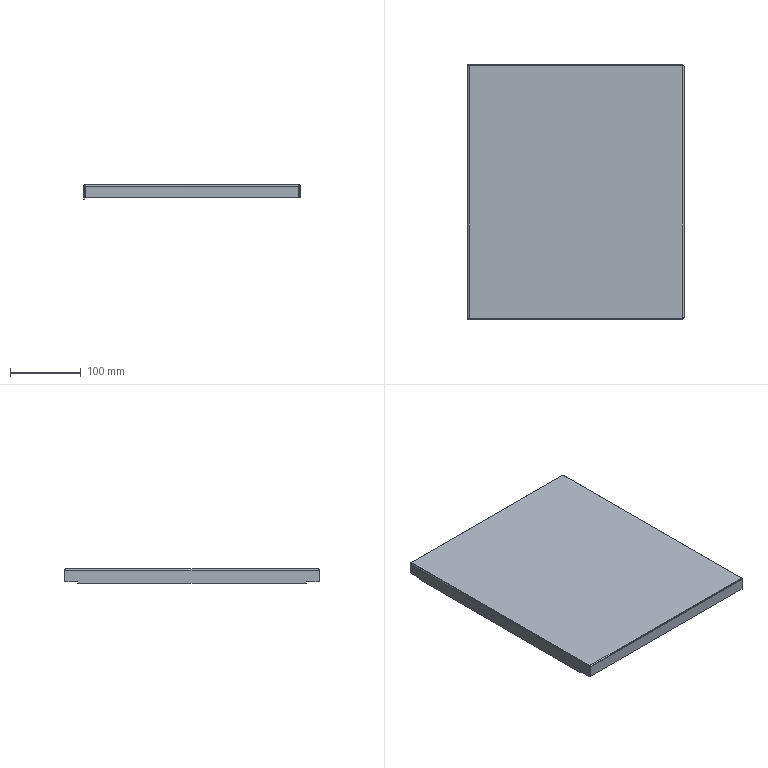Part | SolidWorks | features BaseBody 1 | 1 solid | 44 faces | box 304.9 x 358.65 x 20 mm | volume 157769 mm3 | plane 32 | cylinder 8 | spline 4 | commonest cylinder face diameters 1 x4 3.4 x4
STEP:
#1=CARTESIAN_POINT('',(-152.45,-179.325,-18.));
#2=VERTEX_POINT('',#1);
#3=CARTESIAN_POINT('',(-152.45,-161.325,-18.));
#4=VERTEX_POINT('',#3);
#5=CARTESIAN_POINT('',(-152.45,-179.325,-18.));
#6=DIRECTION('',(0.,1.,0.));
#7=VECTOR('',#6,1000.);
#8=LINE('',#5,#7);
#9=EDGE_CURVE('',#2,#4,#8,.T.);
#10=ORIENTED_EDGE('',*,*,#9,.T.);
#11=CARTESIAN_POINT('',(-151.25,-161.325,-18.));
#12=VERTEX_POINT('',#11);
#13=CARTESIAN_POINT('',(-151.25,-161.325,-18.));
#14=DIRECTION('',(-1.,0.,0.));
#15=VECTOR('',#14,1000.);
#16=LINE('',#13,#15);
#17=EDGE_CURVE('',#12,#4,#16,.T.);
#18=ORIENTED_EDGE('',*,*,#17,.F.);
#19=CARTESIAN_POINT('',(-151.25,-179.325,-18.));
#20=VERTEX_POINT('',#19);
#21=CARTESIAN_POINT('',(-151.25,-179.325,-18.));
#22=DIRECTION('',(0.,1.,0.));
#23=VECTOR('',#22,1000.);
#24=LINE('',#21,#23);
#25=EDGE_CURVE('',#20,#12,#24,.T.);
#26=ORIENTED_EDGE('',*,*,#25,.F.);
#27=CARTESIAN_POINT('',(-151.25,-179.325,-18.));
#28=DIRECTION('',(-1.,0.,0.));
#29=VECTOR('',#28,1000.);
#30=LINE('',#27,#29);
#31=EDGE_CURVE('',#20,#2,#30,.T.);
#32=ORIENTED_EDGE('',*,*,#31,.T.);
#33=EDGE_LOOP('',(#10,#18,#26,#32));
#34=FACE_OUTER_BOUND('',#33,.T.);
#35=CARTESIAN_POINT('',(-151.25,-179.325,-18.));
#36=DIRECTION('',(0.,0.,1.));
#37=DIRECTION('',(1.,0.,0.));
#38=AXIS2_PLACEMENT_3D('',#35,#36,#37);
#39=PLANE('',#38);
#40=ADVANCED_FACE('',(#34),#39,.F.);
#41=CARTESIAN_POINT('',(-152.45,-161.325,-20.));
#42=VERTEX_POINT('',#41);
#43=CARTESIAN_POINT('',(-152.45,-161.325,-20.));
#44=DIRECTION('',(0.,0.,-1.));
#45=VECTOR('',#44,1000.);
#46=LINE('',#43,#45);
#47=EDGE_CURVE('',#4,#42,#46,.T.);
#48=ORIENTED_EDGE('',*,*,#47,.T.);
#49=CARTESIAN_POINT('',(-151.25,-161.325,-20.));
#50=VERTEX_POINT('',#49);
#51=CARTESIAN_POINT('',(-151.25,-161.325,-20.));
#52=DIRECTION('',(-1.,0.,0.));
#53=VECTOR('',#52,1000.);
#54=LINE('',#51,#53);
#55=EDGE_CURVE('',#50,#42,#54,.T.);
#56=ORIENTED_EDGE('',*,*,#55,.F.);
#57=CARTESIAN_POINT('',(-151.25,-161.325,-20.));
#58=DIRECTION('',(0.,0.,-1.));
#59=VECTOR('',#58,1000.);
#60=LINE('',#57,#59);
#61=EDGE_CURVE('',#12,#50,#60,.T.);
#62=ORIENTED_EDGE('',*,*,#61,.F.);
#63=ORIENTED_EDGE('',*,*,#17,.T.);
#64=EDGE_LOOP('',(#48,#56,#62,#63));
#65=FACE_OUTER_BOUND('',#64,.T.);
#66=CARTESIAN_POINT('',(-151.25,-161.325,-20.));
#67=DIRECTION('',(0.,1.,0.));
#68=DIRECTION('',(1.,0.,0.));
#69=AXIS2_PLACEMENT_3D('',#66,#67,#68);
#70=PLANE('',#69);
#71=ADVANCED_FACE('',(#65),#70,.F.);
#72=CARTESIAN_POINT('',(-152.45,161.325,-20.));
#73=VERTEX_POINT('',#72);
#74=CARTESIAN_POINT('',(-152.45,161.325,-18.));
#75=VERTEX_POINT('',#74);
#76=CARTESIAN_POINT('',(-152.45,161.325,-20.));
#77=DIRECTION('',(0.,0.,1.));
#78=VECTOR('',#77,1000.);
#79=LINE('',#76,#78);
#80=EDGE_CURVE('',#73,#75,#79,.T.);
#81=ORIENTED_EDGE('',*,*,#80,.T.);
#82=CARTESIAN_POINT('',(-151.25,161.325,-18.));
#83=VERTEX_POINT('',#82);
#84=CARTESIAN_POINT('',(-151.25,161.325,-18.));
#85=DIRECTION('',(-1.,0.,0.));
#86=VECTOR('',#85,1000.);
#87=LINE('',#84,#86);
#88=EDGE_CURVE('',#83,#75,#87,.T.);
#89=ORIENTED_EDGE('',*,*,#88,.F.);
#90=CARTESIAN_POINT('',(-151.25,161.325,-20.));
#91=VERTEX_POINT('',#90);
#92=CARTESIAN_POINT('',(-151.25,161.325,-20.));
#93=DIRECTION('',(0.,0.,1.));
#94=VECTOR('',#93,1000.);
#95=LINE('',#92,#94);
#96=EDGE_CURVE('',#91,#83,#95,.T.);
#97=ORIENTED_EDGE('',*,*,#96,.F.);
#98=CARTESIAN_POINT('',(-151.25,161.325,-20.));
#99=DIRECTION('',(-1.,0.,0.));
#100=VECTOR('',#99,1000.);
#101=LINE('',#98,#100);
#102=EDGE_CURVE('',#91,#73,#101,.T.);
#103=ORIENTED_EDGE('',*,*,#102,.T.);
#104=EDGE_LOOP('',(#81,#89,#97,#103));
#105=FACE_OUTER_BOUND('',#104,.T.);
#106=CARTESIAN_POINT('',(-151.25,161.325,-20.));
#107=DIRECTION('',(0.,-1.,0.));
#108=DIRECTION('',(0.,0.,-1.));
#109=AXIS2_PLACEMENT_3D('',#106,#107,#108);
#110=PLANE('',#109);
#111=ADVANCED_FACE('',(#105),#110,.F.);
#112=CARTESIAN_POINT('',(-152.45,179.325,-18.));
#113=VERTEX_POINT('',#112);
#114=CARTESIAN_POINT('',(-152.45,179.325,-18.));
#115=DIRECTION('',(0.,1.,0.));
#116=VECTOR('',#115,1000.);
#117=LINE('',#114,#116);
#118=EDGE_CURVE('',#75,#113,#117,.T.);
#119=ORIENTED_EDGE('',*,*,#118,.T.);
#120=CARTESIAN_POINT('',(-151.25,179.325,-18.));
#121=VERTEX_POINT('',#120);
#122=CARTESIAN_POINT('',(-151.25,179.325,-18.));
#123=DIRECTION('',(-1.,0.,0.));
#124=VECTOR('',#123,1000.);
#125=LINE('',#122,#124);
#126=EDGE_CURVE('',#121,#113,#125,.T.);
#127=ORIENTED_EDGE('',*,*,#126,.F.);
#128=CARTESIAN_POINT('',(-151.25,179.325,-18.));
#129=DIRECTION('',(0.,1.,0.));
#130=VECTOR('',#129,1000.);
#131=LINE('',#128,#130);
#132=EDGE_CURVE('',#83,#121,#131,.T.);
#133=ORIENTED_EDGE('',*,*,#132,.F.);
#134=ORIENTED_EDGE('',*,*,#88,.T.);
#135=EDGE_LOOP('',(#119,#127,#133,#134));
#136=FACE_OUTER_BOUND('',#135,.T.);
#137=CARTESIAN_POINT('',(-151.25,179.325,-18.));
#138=DIRECTION('',(0.,0.,1.));
#139=DIRECTION('',(1.,0.,0.));
#140=AXIS2_PLACEMENT_3D('',#137,#138,#139);
#141=PLANE('',#140);
#142=ADVANCED_FACE('',(#136),#141,.F.);
#143=CARTESIAN_POINT('',(150.543,179.325,-18.));
#144=VERTEX_POINT('',#143);
#145=CARTESIAN_POINT('',(150.543,178.125,-18.));
#146=VERTEX_POINT('',#145);
#147=CARTESIAN_POINT('',(150.543,179.325,-18.));
#148=DIRECTION('',(0.,-1.,0.));
#149=VECTOR('',#148,1000.);
#150=LINE('',#147,#149);
#151=EDGE_CURVE('',#144,#146,#150,.T.);
#152=ORIENTED_EDGE('',*,*,#151,.F.);
#153=CARTESIAN_POINT('',(150.543,179.325,-1.7));
#154=VERTEX_POINT('',#153);
#155=CARTESIAN_POINT('',(150.543,179.325,0.));
#156=DIRECTION('',(0.,0.,-1.));
#157=VECTOR('',#156,1000.);
#158=LINE('',#155,#157);
#159=EDGE_CURVE('',#154,#144,#158,.T.);
#160=ORIENTED_EDGE('',*,*,#159,.F.);
#161=CARTESIAN_POINT('',(150.543,178.125,-1.7));
#162=VERTEX_POINT('',#161);
#163=CARTESIAN_POINT('',(150.543,178.125,-1.7));
#164=DIRECTION('',(0.,-1.,0.));
#165=VECTOR('',#164,1000.);
#166=LINE('',#163,#165);
#167=EDGE_CURVE('',#154,#162,#166,.T.);
#168=ORIENTED_EDGE('',*,*,#167,.T.);
#169=CARTESIAN_POINT('',(150.543,178.125,-1.2));
#170=DIRECTION('',(0.,0.,-1.));
#171=VECTOR('',#170,1000.);
#172=LINE('',#169,#171);
#173=EDGE_CURVE('',#162,#146,#172,.T.);
#174=ORIENTED_EDGE('',*,*,#173,.T.);
#175=EDGE_LOOP('',(#152,#160,#168,#174));
#176=FACE_OUTER_BOUND('',#175,.T.);
#177=CARTESIAN_POINT('',(150.543,178.125,-1.2));
#178=DIRECTION('',(-1.,0.,0.));
#179=DIRECTION('',(0.,0.,1.));
#180=AXIS2_PLACEMENT_3D('',#177,#178,#179);
#181=PLANE('',#180);
#182=ADVANCED_FACE('',(#176),#181,.F.);
#183=CARTESIAN_POINT('',(-150.75,179.325,-18.));
#184=VERTEX_POINT('',#183);
#185=CARTESIAN_POINT('',(0.,179.325,-18.));
#186=DIRECTION('',(-1.,0.,0.));
#187=VECTOR('',#186,1000.);
#188=LINE('',#185,#187);
#189=EDGE_CURVE('',#144,#184,#188,.T.);
#190=ORIENTED_EDGE('',*,*,#189,.F.);
#191=ORIENTED_EDGE('',*,*,#151,.T.);
#192=CARTESIAN_POINT('',(-150.75,178.125,-18.));
#193=VERTEX_POINT('',#192);
#194=CARTESIAN_POINT('',(-150.75,178.125,-18.));
#195=DIRECTION('',(-1.,0.,0.));
#196=VECTOR('',#195,1000.);
#197=LINE('',#194,#196);
#198=EDGE_CURVE('',#146,#193,#197,.T.);
#199=ORIENTED_EDGE('',*,*,#198,.T.);
#200=CARTESIAN_POINT('',(-150.75,179.325,-18.));
#201=DIRECTION('',(0.,-1.,0.));
#202=VECTOR('',#201,1000.);
#203=LINE('',#200,#202);
#204=EDGE_CURVE('',#184,#193,#203,.T.);
#205=ORIENTED_EDGE('',*,*,#204,.F.);
#206=EDGE_LOOP('',(#190,#191,#199,#205));
#207=FACE_OUTER_BOUND('',#206,.T.);
#208=CARTESIAN_POINT('',(-150.75,179.325,-18.));
#209=DIRECTION('',(0.,0.,1.));
#210=DIRECTION('',(0.,-1.,0.));
#211=AXIS2_PLACEMENT_3D('',#208,#209,#210);
#212=PLANE('',#211);
#213=ADVANCED_FACE('',(#207),#212,.F.);
#214=ORIENTED_EDGE('',*,*,#173,.F.);
#215=CARTESIAN_POINT('',(-150.75,178.125,-1.7));
#216=VERTEX_POINT('',#215);
#217=CARTESIAN_POINT('',(-150.75,178.125,-1.7));
#218=DIRECTION('',(1.,0.,0.));
#219=VECTOR('',#218,1000.);
#220=LINE('',#217,#219);
#221=EDGE_CURVE('',#216,#162,#220,.T.);
#222=ORIENTED_EDGE('',*,*,#221,.F.);
#223=CARTESIAN_POINT('',(-150.75,178.125,-1.2));
#224=DIRECTION('',(0.,0.,1.));
#225=VECTOR('',#224,1000.);
#226=LINE('',#223,#225);
#227=EDGE_CURVE('',#193,#216,#226,.T.);
#228=ORIENTED_EDGE('',*,*,#227,.F.);
#229=ORIENTED_EDGE('',*,*,#198,.F.);
#230=EDGE_LOOP('',(#214,#222,#228,#229));
#231=FACE_OUTER_BOUND('',#230,.T.);
#232=CARTESIAN_POINT('',(0.,178.125,0.));
#233=DIRECTION('',(0.,-1.,0.));
#234=DIRECTION('',(0.,0.,-1.));
#235=AXIS2_PLACEMENT_3D('',#232,#233,#234);
#236=PLANE('',#235);
#237=ADVANCED_FACE('',(#231),#236,.T.);
#238=CARTESIAN_POINT('',(-150.75,179.325,-1.7));
#239=VERTEX_POINT('',#238);
#240=CARTESIAN_POINT('',(-150.75,179.325,-1.7));
#241=DIRECTION('',(-1.,0.,0.));
#242=VECTOR('',#241,1000.);
#243=LINE('',#240,#242);
#244=EDGE_CURVE('',#154,#239,#243,.T.);
#245=ORIENTED_EDGE('',*,*,#244,.F.);
#246=ORIENTED_EDGE('',*,*,#159,.T.);
#247=ORIENTED_EDGE('',*,*,#189,.T.);
#248=CARTESIAN_POINT('',(-150.75,179.325,0.));
#249=DIRECTION('',(0.,0.,1.));
#250=VECTOR('',#249,1000.);
#251=LINE('',#248,#250);
#252=EDGE_CURVE('',#184,#239,#251,.T.);
#253=ORIENTED_EDGE('',*,*,#252,.T.);
#254=EDGE_LOOP('',(#245,#246,#247,#253));
#255=FACE_OUTER_BOUND('',#254,.T.);
#256=CARTESIAN_POINT('',(0.,179.325,0.));
#257=DIRECTION('',(0.,-1.,0.));
#258=DIRECTION('',(0.,0.,-1.));
#259=AXIS2_PLACEMENT_3D('',#256,#257,#258);
#260=PLANE('',#259);
#261=ADVANCED_FACE('',(#255),#260,.F.);
#262=CARTESIAN_POINT('',(-150.75,179.325,-1.7));
#263=DIRECTION('',(0.,1.,0.));
#264=VECTOR('',#263,1000.);
#265=LINE('',#262,#264);
#266=EDGE_CURVE('',#216,#239,#265,.T.);
#267=ORIENTED_EDGE('',*,*,#266,.T.);
#268=ORIENTED_EDGE('',*,*,#252,.F.);
#269=ORIENTED_EDGE('',*,*,#204,.T.);
#270=ORIENTED_EDGE('',*,*,#227,.T.);
#271=EDGE_LOOP('',(#267,#268,#269,#270));
#272=FACE_OUTER_BOUND('',#271,.T.);
#273=CARTESIAN_POINT('',(-150.75,179.325,-1.2));
#274=DIRECTION('',(1.,0.,0.));
#275=DIRECTION('',(0.,0.,-1.));
#276=AXIS2_PLACEMENT_3D('',#273,#274,#275);
#277=PLANE('',#276);
#278=ADVANCED_FACE('',(#272),#277,.F.);
#279=CARTESIAN_POINT('',(150.75,177.625,-1.2));
#280=VERTEX_POINT('',#279);
#281=CARTESIAN_POINT('',(-150.75,177.625,-1.2));
#282=VERTEX_POINT('',#281);
#283=CARTESIAN_POINT('',(150.75,177.625,-1.2));
#284=DIRECTION('',(-1.,0.,0.));
#285=VECTOR('',#284,1000.);
#286=LINE('',#283,#285);
#287=EDGE_CURVE('',#280,#282,#286,.T.);
#288=ORIENTED_EDGE('',*,*,#287,.T.);
#289=CARTESIAN_POINT('',(-150.75,177.625,-1.7));
#290=DIRECTION('',(-1.,0.,0.));
#291=DIRECTION('',(0.,0.,-1.));
#292=AXIS2_PLACEMENT_3D('',#289,#290,#291);
#293=CIRCLE('',#292,0.5);
#294=EDGE_CURVE('',#282,#216,#293,.T.);
#295=ORIENTED_EDGE('',*,*,#294,.T.);
#296=ORIENTED_EDGE('',*,*,#221,.T.);
#297=CARTESIAN_POINT('',(150.543,178.125,-1.7));
#298=CARTESIAN_POINT('',(150.577,178.125,-1.569));
#299=CARTESIAN_POINT('',(150.612,178.071,-1.439));
#300=CARTESIAN_POINT('',(150.681,177.886,-1.254));
#301=CARTESIAN_POINT('',(150.715,177.756,-1.2));
#302=CARTESIAN_POINT('',(150.75,177.625,-1.2));
#303=B_SPLINE_CURVE_WITH_KNOTS('',3,(#297,#298,#299,#300,#301,#302),.UNSPECIFIED.,.F.,.F.,(4,2,4),(0.,0.5,1.),.UNSPECIFIED.);
#304=EDGE_CURVE('',#162,#280,#303,.T.);
#305=ORIENTED_EDGE('',*,*,#304,.T.);
#306=EDGE_LOOP('',(#288,#295,#296,#305));
#307=FACE_OUTER_BOUND('',#306,.T.);
#308=CARTESIAN_POINT('',(150.75,177.625,-1.7));
#309=DIRECTION('',(1.,0.,0.));
#310=DIRECTION('',(0.,1.,0.));
#311=AXIS2_PLACEMENT_3D('',#308,#309,#310);
#312=CYLINDRICAL_SURFACE('',#311,0.5);
#313=ADVANCED_FACE('',(#307),#312,.F.);
#314=CARTESIAN_POINT('',(150.75,177.625,0.));
#315=VERTEX_POINT('',#314);
#316=CARTESIAN_POINT('',(-150.75,177.625,0.));
#317=VERTEX_POINT('',#316);
#318=CARTESIAN_POINT('',(150.75,177.625,0.));
#319=DIRECTION('',(-1.,0.,0.));
#320=VECTOR('',#319,1000.);
#321=LINE('',#318,#320);
#322=EDGE_CURVE('',#315,#317,#321,.T.);
#323=ORIENTED_EDGE('',*,*,#322,.F.);
#324=CARTESIAN_POINT('',(150.543,179.325,-1.7));
#325=CARTESIAN_POINT('',(150.56,179.325,-1.477));
#326=CARTESIAN_POINT('',(150.577,179.281,-1.255));
#327=CARTESIAN_POINT('',(150.612,179.11,-0.8438));
#328=CARTESIAN_POINT('',(150.629,178.984,-0.6553));
#329=CARTESIAN_POINT('',(150.664,178.67,-0.3406));
#330=CARTESIAN_POINT('',(150.681,178.481,-0.2146));
#331=CARTESIAN_POINT('',(150.715,178.07,-0.04425));
#332=CARTESIAN_POINT('',(150.733,177.848,0.));
#333=CARTESIAN_POINT('',(150.75,177.625,0.));
#334=B_SPLINE_CURVE_WITH_KNOTS('',3,(#324,#325,#326,#327,#328,#329,#330,#331,#332,#333),.UNSPECIFIED.,.F.,.F.,(4,2,2,2,4),(0.,0.25,0.5,0.75,1.),.UNSPECIFIED.);
#335=EDGE_CURVE('',#154,#315,#334,.T.);
#336=ORIENTED_EDGE('',*,*,#335,.F.);
#337=ORIENTED_EDGE('',*,*,#244,.T.);
#338=CARTESIAN_POINT('',(-150.75,177.625,-1.7));
#339=DIRECTION('',(-1.,0.,0.));
#340=DIRECTION('',(0.,0.,-1.));
#341=AXIS2_PLACEMENT_3D('',#338,#339,#340);
#342=CIRCLE('',#341,1.7);
#343=EDGE_CURVE('',#317,#239,#342,.T.);
#344=ORIENTED_EDGE('',*,*,#343,.F.);
#345=EDGE_LOOP('',(#323,#336,#337,#344));
#346=FACE_OUTER_BOUND('',#345,.T.);
#347=CARTESIAN_POINT('',(150.75,177.625,-1.7));
#348=DIRECTION('',(1.,0.,0.));
#349=DIRECTION('',(0.,1.,0.));
#350=AXIS2_PLACEMENT_3D('',#347,#348,#349);
#351=CYLINDRICAL_SURFACE('',#350,1.7);
#352=ADVANCED_FACE('',(#346),#351,.T.);
#353=ORIENTED_EDGE('',*,*,#304,.F.);
#354=ORIENTED_EDGE('',*,*,#167,.F.);
#355=ORIENTED_EDGE('',*,*,#335,.T.);
#356=CARTESIAN_POINT('',(150.75,177.625,-1.2));
#357=DIRECTION('',(0.,0.,1.));
#358=VECTOR('',#357,1000.);
#359=LINE('',#356,#358);
#360=EDGE_CURVE('',#280,#315,#359,.T.);
#361=ORIENTED_EDGE('',*,*,#360,.F.);
#362=EDGE_LOOP('',(#353,#354,#355,#361));
#363=FACE_OUTER_BOUND('',#362,.T.);
#364=CARTESIAN_POINT('',(150.543,179.337,-1.7));
#365=CARTESIAN_POINT('',(150.56,179.337,-1.476));
#366=CARTESIAN_POINT('',(150.577,179.292,-1.252));
#367=CARTESIAN_POINT('',(150.612,179.121,-0.8378));
#368=CARTESIAN_POINT('',(150.629,178.994,-0.6479));
#369=CARTESIAN_POINT('',(150.664,178.677,-0.331));
#370=CARTESIAN_POINT('',(150.681,178.487,-0.2041));
#371=CARTESIAN_POINT('',(150.715,178.073,-0.03256));
#372=CARTESIAN_POINT('',(150.733,177.849,0.012));
#373=CARTESIAN_POINT('',(150.75,177.625,0.012));
#374=CARTESIAN_POINT('',(150.543,179.325,-1.7));
#375=CARTESIAN_POINT('',(150.56,179.325,-1.477));
#376=CARTESIAN_POINT('',(150.577,179.281,-1.255));
#377=CARTESIAN_POINT('',(150.612,179.11,-0.8438));
#378=CARTESIAN_POINT('',(150.629,178.984,-0.6553));
#379=CARTESIAN_POINT('',(150.664,178.67,-0.3406));
#380=CARTESIAN_POINT('',(150.681,178.481,-0.2146));
#381=CARTESIAN_POINT('',(150.715,178.07,-0.04425));
#382=CARTESIAN_POINT('',(150.733,177.848,0.));
#383=CARTESIAN_POINT('',(150.75,177.625,0.));
#384=CARTESIAN_POINT('',(150.543,178.125,-1.7));
#385=CARTESIAN_POINT('',(150.56,178.125,-1.635));
#386=CARTESIAN_POINT('',(150.577,178.112,-1.569));
#387=CARTESIAN_POINT('',(150.612,178.062,-1.448));
#388=CARTESIAN_POINT('',(150.629,178.025,-1.393));
#389=CARTESIAN_POINT('',(150.664,177.932,-1.3));
#390=CARTESIAN_POINT('',(150.681,177.877,-1.263));
#391=CARTESIAN_POINT('',(150.715,177.756,-1.213));
#392=CARTESIAN_POINT('',(150.733,177.69,-1.2));
#393=CARTESIAN_POINT('',(150.75,177.625,-1.2));
#394=CARTESIAN_POINT('',(150.543,178.113,-1.7));
#395=CARTESIAN_POINT('',(150.56,178.113,-1.636));
#396=CARTESIAN_POINT('',(150.577,178.1,-1.572));
#397=CARTESIAN_POINT('',(150.612,178.051,-1.454));
#398=CARTESIAN_POINT('',(150.629,178.015,-1.4));
#399=CARTESIAN_POINT('',(150.664,177.925,-1.31));
#400=CARTESIAN_POINT('',(150.681,177.871,-1.274));
#401=CARTESIAN_POINT('',(150.715,177.753,-1.225));
#402=CARTESIAN_POINT('',(150.733,177.689,-1.212));
#403=CARTESIAN_POINT('',(150.75,177.625,-1.212));
#404=B_SPLINE_SURFACE_WITH_KNOTS('',1,3,((#364,#365,#366,#367,#368,#369,#370,#371,#372,#373),(#374,#375,#376,#377,#378,#379,#380,#381,#382,#383),(#384,#385,#386,#387,#388,#389,#390,#391,#392,#393),(#394,#395,#396,#397,#398,#399,#400,#401,#402,#403)),.UNSPECIFIED.,.F.,.F.,.F.,(2,1,1,2),(4,2,2,2,4),(-0.01,0.,1.,1.01),(0.,0.25,0.5,0.75,1.),.UNSPECIFIED.);
#405=ADVANCED_FACE('',(#363),#404,.F.);
#406=ORIENTED_EDGE('',*,*,#266,.F.);
#407=ORIENTED_EDGE('',*,*,#294,.F.);
#408=CARTESIAN_POINT('',(-150.75,177.625,-1.2));
#409=DIRECTION('',(0.,0.,1.));
#410=VECTOR('',#409,1000.);
#411=LINE('',#408,#410);
#412=EDGE_CURVE('',#282,#317,#411,.T.);
#413=ORIENTED_EDGE('',*,*,#412,.T.);
#414=ORIENTED_EDGE('',*,*,#343,.T.);
#415=EDGE_LOOP('',(#406,#407,#413,#414));
#416=FACE_OUTER_BOUND('',#415,.T.);
#417=CARTESIAN_POINT('',(-150.75,177.625,-1.7));
#418=DIRECTION('',(-1.,0.,0.));
#419=DIRECTION('',(0.,0.,1.));
#420=AXIS2_PLACEMENT_3D('',#417,#418,#419);
#421=PLANE('',#420);
#422=ADVANCED_FACE('',(#416),#421,.T.);
#423=CARTESIAN_POINT('',(152.45,-177.418,-18.));
#424=VERTEX_POINT('',#423);
#425=CARTESIAN_POINT('',(151.25,-177.418,-18.));
#426=VERTEX_POINT('',#425);
#427=CARTESIAN_POINT('',(152.45,-177.418,-18.));
#428=DIRECTION('',(-1.,0.,0.));
#429=VECTOR('',#428,1000.);
#430=LINE('',#427,#429);
#431=EDGE_CURVE('',#424,#426,#430,.T.);
#432=ORIENTED_EDGE('',*,*,#431,.F.);
#433=CARTESIAN_POINT('',(152.45,-177.418,-1.7));
#434=VERTEX_POINT('',#433);
#435=CARTESIAN_POINT('',(152.45,-177.418,0.));
#436=DIRECTION('',(0.,0.,-1.));
#437=VECTOR('',#436,1000.);
#438=LINE('',#435,#437);
#439=EDGE_CURVE('',#434,#424,#438,.T.);
#440=ORIENTED_EDGE('',*,*,#439,.F.);
#441=CARTESIAN_POINT('',(151.25,-177.418,-1.7));
#442=VERTEX_POINT('',#441);
#443=CARTESIAN_POINT('',(151.25,-177.418,-1.7));
#444=DIRECTION('',(-1.,0.,0.));
#445=VECTOR('',#444,1000.);
#446=LINE('',#443,#445);
#447=EDGE_CURVE('',#434,#442,#446,.T.);
#448=ORIENTED_EDGE('',*,*,#447,.T.);
#449=CARTESIAN_POINT('',(151.25,-177.418,-1.2));
#450=DIRECTION('',(0.,0.,-1.));
#451=VECTOR('',#450,1000.);
#452=LINE('',#449,#451);
#453=EDGE_CURVE('',#442,#426,#452,.T.);
#454=ORIENTED_EDGE('',*,*,#453,.T.);
#455=EDGE_LOOP('',(#432,#440,#448,#454));
#456=FACE_OUTER_BOUND('',#455,.T.);
#457=CARTESIAN_POINT('',(151.25,-177.418,-1.2));
#458=DIRECTION('',(0.,1.,0.));
#459=DIRECTION('',(0.,0.,-1.));
#460=AXIS2_PLACEMENT_3D('',#457,#458,#459);
#461=PLANE('',#460);
#462=ADVANCED_FACE('',(#456),#461,.F.);
#463=CARTESIAN_POINT('',(152.45,177.418,-18.));
#464=VERTEX_POINT('',#463);
#465=CARTESIAN_POINT('',(151.25,177.418,-18.));
#466=VERTEX_POINT('',#465);
#467=CARTESIAN_POINT('',(151.25,177.418,-18.));
#468=DIRECTION('',(-1.,0.,0.));
#469=VECTOR('',#468,1000.);
#470=LINE('',#467,#469);
#471=EDGE_CURVE('',#464,#466,#470,.T.);
#472=ORIENTED_EDGE('',*,*,#471,.F.);
#473=CARTESIAN_POINT('',(152.45,0.,-18.));
#474=DIRECTION('',(0.,1.,0.));
#475=VECTOR('',#474,1000.);
#476=LINE('',#473,#475);
#477=EDGE_CURVE('',#424,#464,#476,.T.);
#478=ORIENTED_EDGE('',*,*,#477,.F.);
#479=ORIENTED_EDGE('',*,*,#431,.T.);
#480=CARTESIAN_POINT('',(151.25,179.325,-18.));
#481=DIRECTION('',(0.,1.,0.));
#482=VECTOR('',#481,1000.);
#483=LINE('',#480,#482);
#484=EDGE_CURVE('',#426,#466,#483,.T.);
#485=ORIENTED_EDGE('',*,*,#484,.T.);
#486=EDGE_LOOP('',(#472,#478,#479,#485));
#487=FACE_OUTER_BOUND('',#486,.T.);
#488=CARTESIAN_POINT('',(152.45,179.325,-18.));
#489=DIRECTION('',(0.,0.,1.));
#490=DIRECTION('',(1.,0.,0.));
#491=AXIS2_PLACEMENT_3D('',#488,#489,#490);
#492=PLANE('',#491);
#493=ADVANCED_FACE('',(#487),#492,.F.);
#494=CARTESIAN_POINT('',(151.25,177.418,-1.7));
#495=VERTEX_POINT('',#494);
#496=CARTESIAN_POINT('',(151.25,179.325,-1.7));
#497=DIRECTION('',(0.,-1.,0.));
#498=VECTOR('',#497,1000.);
#499=LINE('',#496,#498);
#500=EDGE_CURVE('',#495,#442,#499,.T.);
#501=ORIENTED_EDGE('',*,*,#500,.F.);
#502=CARTESIAN_POINT('',(151.25,177.418,0.));
#503=DIRECTION('',(0.,0.,-1.));
#504=VECTOR('',#503,1000.);
#505=LINE('',#502,#504);
#506=EDGE_CURVE('',#495,#466,#505,.T.);
#507=ORIENTED_EDGE('',*,*,#506,.T.);
#508=ORIENTED_EDGE('',*,*,#484,.F.);
#509=ORIENTED_EDGE('',*,*,#453,.F.);
#510=EDGE_LOOP('',(#501,#507,#508,#509));
#511=FACE_OUTER_BOUND('',#510,.T.);
#512=CARTESIAN_POINT('',(151.25,0.,0.));
#513=DIRECTION('',(-1.,0.,0.));
#514=DIRECTION('',(0.,0.,1.));
#515=AXIS2_PLACEMENT_3D('',#512,#513,#514);
#516=PLANE('',#515);
#517=ADVANCED_FACE('',(#511),#516,.T.);
#518=CARTESIAN_POINT('',(152.45,177.418,-1.7));
#519=VERTEX_POINT('',#518);
#520=CARTESIAN_POINT('',(152.45,177.418,-1.2));
#521=DIRECTION('',(0.,0.,-1.));
#522=VECTOR('',#521,1000.);
#523=LINE('',#520,#522);
#524=EDGE_CURVE('',#519,#464,#523,.T.);
#525=ORIENTED_EDGE('',*,*,#524,.F.);
#526=CARTESIAN_POINT('',(152.45,179.325,-1.7));
#527=DIRECTION('',(0.,1.,0.));
#528=VECTOR('',#527,1000.);
#529=LINE('',#526,#528);
#530=EDGE_CURVE('',#434,#519,#529,.T.);
#531=ORIENTED_EDGE('',*,*,#530,.F.);
#532=ORIENTED_EDGE('',*,*,#439,.T.);
#533=ORIENTED_EDGE('',*,*,#477,.T.);
#534=EDGE_LOOP('',(#525,#531,#532,#533));
#535=FACE_OUTER_BOUND('',#534,.T.);
#536=CARTESIAN_POINT('',(152.45,0.,0.));
#537=DIRECTION('',(-1.,0.,0.));
#538=DIRECTION('',(0.,0.,1.));
#539=AXIS2_PLACEMENT_3D('',#536,#537,#538);
#540=PLANE('',#539);
#541=ADVANCED_FACE('',(#535),#540,.F.);
#542=ORIENTED_EDGE('',*,*,#524,.T.);
#543=ORIENTED_EDGE('',*,*,#471,.T.);
#544=ORIENTED_EDGE('',*,*,#506,.F.);
#545=CARTESIAN_POINT('',(151.25,177.418,-1.7));
#546=DIRECTION('',(-1.,0.,0.));
#547=VECTOR('',#546,1000.);
#548=LINE('',#545,#547);
#549=EDGE_CURVE('',#519,#495,#548,.T.);
#550=ORIENTED_EDGE('',*,*,#549,.F.);
#551=EDGE_LOOP('',(#542,#543,#544,#550));
#552=FACE_OUTER_BOUND('',#551,.T.);
#553=CARTESIAN_POINT('',(151.25,177.418,-1.2));
#554=DIRECTION('',(0.,1.,0.));
#555=DIRECTION('',(0.,0.,-1.));
#556=AXIS2_PLACEMENT_3D('',#553,#554,#555);
#557=PLANE('',#556);
#558=ADVANCED_FACE('',(#552),#557,.T.);
#559=CARTESIAN_POINT('',(150.75,-177.625,-1.2));
#560=VERTEX_POINT('',#559);
#561=CARTESIAN_POINT('',(150.75,-177.625,-1.2));
#562=DIRECTION('',(0.,1.,0.));
#563=VECTOR('',#562,1000.);
#564=LINE('',#561,#563);
#565=EDGE_CURVE('',#560,#280,#564,.T.);
#566=ORIENTED_EDGE('',*,*,#565,.T.);
#567=CARTESIAN_POINT('',(150.75,177.625,-1.2));
#568=CARTESIAN_POINT('',(150.881,177.59,-1.2));
#569=CARTESIAN_POINT('',(151.011,177.556,-1.254));
#570=CARTESIAN_POINT('',(151.196,177.487,-1.439));
#571=CARTESIAN_POINT('',(151.25,177.452,-1.569));
#572=CARTESIAN_POINT('',(151.25,177.418,-1.7));
#573=B_SPLINE_CURVE_WITH_KNOTS('',3,(#567,#568,#569,#570,#571,#572),.UNSPECIFIED.,.F.,.F.,(4,2,4),(0.,0.5,1.),.UNSPECIFIED.);
#574=EDGE_CURVE('',#280,#495,#573,.T.);
#575=ORIENTED_EDGE('',*,*,#574,.T.);
#576=ORIENTED_EDGE('',*,*,#500,.T.);
#577=CARTESIAN_POINT('',(151.25,-177.418,-1.7));
#578=CARTESIAN_POINT('',(151.25,-177.452,-1.569));
#579=CARTESIAN_POINT('',(151.196,-177.487,-1.439));
#580=CARTESIAN_POINT('',(151.011,-177.556,-1.254));
#581=CARTESIAN_POINT('',(150.881,-177.59,-1.2));
#582=CARTESIAN_POINT('',(150.75,-177.625,-1.2));
#583=B_SPLINE_CURVE_WITH_KNOTS('',3,(#577,#578,#579,#580,#581,#582),.UNSPECIFIED.,.F.,.F.,(4,2,4),(0.,0.5,1.),.UNSPECIFIED.);
#584=EDGE_CURVE('',#442,#560,#583,.T.);
#585=ORIENTED_EDGE('',*,*,#584,.T.);
#586=EDGE_LOOP('',(#566,#575,#576,#585));
#587=FACE_OUTER_BOUND('',#586,.T.);
#588=CARTESIAN_POINT('',(150.75,-177.625,-1.7));
#589=DIRECTION('',(0.,-1.,0.));
#590=DIRECTION('',(1.,0.,0.));
#591=AXIS2_PLACEMENT_3D('',#588,#589,#590);
#592=CYLINDRICAL_SURFACE('',#591,0.5);
#593=ADVANCED_FACE('',(#587),#592,.F.);
#594=CARTESIAN_POINT('',(150.75,-177.625,0.));
#595=VERTEX_POINT('',#594);
#596=CARTESIAN_POINT('',(150.75,-177.625,0.));
#597=DIRECTION('',(0.,1.,0.));
#598=VECTOR('',#597,1000.);
#599=LINE('',#596,#598);
#600=EDGE_CURVE('',#595,#315,#599,.T.);
#601=ORIENTED_EDGE('',*,*,#600,.F.);
#602=CARTESIAN_POINT('',(152.45,-177.418,-1.7));
#603=CARTESIAN_POINT('',(152.45,-177.435,-1.477));
#604=CARTESIAN_POINT('',(152.406,-177.452,-1.255));
#605=CARTESIAN_POINT('',(152.235,-177.487,-0.8438));
#606=CARTESIAN_POINT('',(152.109,-177.504,-0.6553));
#607=CARTESIAN_POINT('',(151.795,-177.539,-0.3406));
#608=CARTESIAN_POINT('',(151.606,-177.556,-0.2146));
#609=CARTESIAN_POINT('',(151.195,-177.59,-0.04425));
#610=CARTESIAN_POINT('',(150.973,-177.608,0.));
#611=CARTESIAN_POINT('',(150.75,-177.625,0.));
#612=B_SPLINE_CURVE_WITH_KNOTS('',3,(#602,#603,#604,#605,#606,#607,#608,#609,#610,#611),.UNSPECIFIED.,.F.,.F.,(4,2,2,2,4),(0.,0.25,0.5,0.75,1.),.UNSPECIFIED.);
#613=EDGE_CURVE('',#434,#595,#612,.T.);
#614=ORIENTED_EDGE('',*,*,#613,.F.);
#615=ORIENTED_EDGE('',*,*,#530,.T.);
#616=CARTESIAN_POINT('',(150.75,177.625,0.));
#617=CARTESIAN_POINT('',(150.973,177.608,0.));
#618=CARTESIAN_POINT('',(151.195,177.59,-0.04425));
#619=CARTESIAN_POINT('',(151.606,177.556,-0.2146));
#620=CARTESIAN_POINT('',(151.795,177.539,-0.3406));
#621=CARTESIAN_POINT('',(152.109,177.504,-0.6553));
#622=CARTESIAN_POINT('',(152.235,177.487,-0.8438));
#623=CARTESIAN_POINT('',(152.406,177.452,-1.255));
#624=CARTESIAN_POINT('',(152.45,177.435,-1.477));
#625=CARTESIAN_POINT('',(152.45,177.418,-1.7));
#626=B_SPLINE_CURVE_WITH_KNOTS('',3,(#616,#617,#618,#619,#620,#621,#622,#623,#624,#625),.UNSPECIFIED.,.F.,.F.,(4,2,2,2,4),(0.,0.25,0.5,0.75,1.),.UNSPECIFIED.);
#627=EDGE_CURVE('',#315,#519,#626,.T.);
#628=ORIENTED_EDGE('',*,*,#627,.F.);
#629=EDGE_LOOP('',(#601,#614,#615,#628));
#630=FACE_OUTER_BOUND('',#629,.T.);
#631=CARTESIAN_POINT('',(150.75,-177.625,-1.7));
#632=DIRECTION('',(0.,-1.,0.));
#633=DIRECTION('',(1.,0.,0.));
#634=AXIS2_PLACEMENT_3D('',#631,#632,#633);
#635=CYLINDRICAL_SURFACE('',#634,1.7);
#636=ADVANCED_FACE('',(#630),#635,.T.);
#637=ORIENTED_EDGE('',*,*,#584,.F.);
#638=ORIENTED_EDGE('',*,*,#447,.F.);
#639=ORIENTED_EDGE('',*,*,#613,.T.);
#640=CARTESIAN_POINT('',(150.75,-177.625,-1.2));
#641=DIRECTION('',(0.,0.,1.));
#642=VECTOR('',#641,1000.);
#643=LINE('',#640,#642);
#644=EDGE_CURVE('',#560,#595,#643,.T.);
#645=ORIENTED_EDGE('',*,*,#644,.F.);
#646=EDGE_LOOP('',(#637,#638,#639,#645));
#647=FACE_OUTER_BOUND('',#646,.T.);
#648=CARTESIAN_POINT('',(152.462,-177.418,-1.7));
#649=CARTESIAN_POINT('',(152.462,-177.435,-1.476));
#650=CARTESIAN_POINT('',(152.417,-177.452,-1.252));
#651=CARTESIAN_POINT('',(152.246,-177.487,-0.8378));
#652=CARTESIAN_POINT('',(152.119,-177.504,-0.6479));
#653=CARTESIAN_POINT('',(151.802,-177.539,-0.331));
#654=CARTESIAN_POINT('',(151.612,-177.556,-0.2041));
#655=CARTESIAN_POINT('',(151.198,-177.59,-0.03256));
#656=CARTESIAN_POINT('',(150.974,-177.608,0.012));
#657=CARTESIAN_POINT('',(150.75,-177.625,0.012));
#658=CARTESIAN_POINT('',(152.45,-177.418,-1.7));
#659=CARTESIAN_POINT('',(152.45,-177.435,-1.477));
#660=CARTESIAN_POINT('',(152.406,-177.452,-1.255));
#661=CARTESIAN_POINT('',(152.235,-177.487,-0.8438));
#662=CARTESIAN_POINT('',(152.109,-177.504,-0.6553));
#663=CARTESIAN_POINT('',(151.795,-177.539,-0.3406));
#664=CARTESIAN_POINT('',(151.606,-177.556,-0.2146));
#665=CARTESIAN_POINT('',(151.195,-177.59,-0.04425));
#666=CARTESIAN_POINT('',(150.973,-177.608,0.));
#667=CARTESIAN_POINT('',(150.75,-177.625,0.));
#668=CARTESIAN_POINT('',(151.25,-177.418,-1.7));
#669=CARTESIAN_POINT('',(151.25,-177.435,-1.635));
#670=CARTESIAN_POINT('',(151.237,-177.452,-1.569));
#671=CARTESIAN_POINT('',(151.187,-177.487,-1.448));
#672=CARTESIAN_POINT('',(151.15,-177.504,-1.393));
#673=CARTESIAN_POINT('',(151.057,-177.539,-1.3));
#674=CARTESIAN_POINT('',(151.002,-177.556,-1.263));
#675=CARTESIAN_POINT('',(150.881,-177.59,-1.213));
#676=CARTESIAN_POINT('',(150.815,-177.608,-1.2));
#677=CARTESIAN_POINT('',(150.75,-177.625,-1.2));
#678=CARTESIAN_POINT('',(151.238,-177.418,-1.7));
#679=CARTESIAN_POINT('',(151.238,-177.435,-1.636));
#680=CARTESIAN_POINT('',(151.225,-177.452,-1.572));
#681=CARTESIAN_POINT('',(151.176,-177.487,-1.454));
#682=CARTESIAN_POINT('',(151.14,-177.504,-1.4));
#683=CARTESIAN_POINT('',(151.05,-177.539,-1.31));
#684=CARTESIAN_POINT('',(150.996,-177.556,-1.274));
#685=CARTESIAN_POINT('',(150.878,-177.59,-1.225));
#686=CARTESIAN_POINT('',(150.814,-177.608,-1.212));
#687=CARTESIAN_POINT('',(150.75,-177.625,-1.212));
#688=B_SPLINE_SURFACE_WITH_KNOTS('',1,3,((#648,#649,#650,#651,#652,#653,#654,#655,#656,#657),(#658,#659,#660,#661,#662,#663,#664,#665,#666,#667),(#668,#669,#670,#671,#672,#673,#674,#675,#676,#677),(#678,#679,#680,#681,#682,#683,#684,#685,#686,#687)),.UNSPECIFIED.,.F.,.F.,.F.,(2,1,1,2),(4,2,2,2,4),(-0.01,0.,1.,1.01),(0.,0.25,0.5,0.75,1.),.UNSPECIFIED.);
#689=ADVANCED_FACE('',(#647),#688,.F.);
#690=ORIENTED_EDGE('',*,*,#549,.T.);
#691=ORIENTED_EDGE('',*,*,#574,.F.);
#692=ORIENTED_EDGE('',*,*,#360,.T.);
#693=ORIENTED_EDGE('',*,*,#627,.T.);
#694=EDGE_LOOP('',(#690,#691,#692,#693));
#695=FACE_OUTER_BOUND('',#694,.T.);
#696=CARTESIAN_POINT('',(150.75,177.625,0.012));
#697=CARTESIAN_POINT('',(150.974,177.608,0.012));
#698=CARTESIAN_POINT('',(151.198,177.59,-0.03256));
#699=CARTESIAN_POINT('',(151.612,177.556,-0.2041));
#700=CARTESIAN_POINT('',(151.802,177.539,-0.331));
#701=CARTESIAN_POINT('',(152.119,177.504,-0.6479));
#702=CARTESIAN_POINT('',(152.246,177.487,-0.8378));
#703=CARTESIAN_POINT('',(152.417,177.452,-1.252));
#704=CARTESIAN_POINT('',(152.462,177.435,-1.476));
#705=CARTESIAN_POINT('',(152.462,177.418,-1.7));
#706=CARTESIAN_POINT('',(150.75,177.625,0.));
#707=CARTESIAN_POINT('',(150.973,177.608,0.));
#708=CARTESIAN_POINT('',(151.195,177.59,-0.04425));
#709=CARTESIAN_POINT('',(151.606,177.556,-0.2146));
#710=CARTESIAN_POINT('',(151.795,177.539,-0.3406));
#711=CARTESIAN_POINT('',(152.109,177.504,-0.6553));
#712=CARTESIAN_POINT('',(152.235,177.487,-0.8438));
#713=CARTESIAN_POINT('',(152.406,177.452,-1.255));
#714=CARTESIAN_POINT('',(152.45,177.435,-1.477));
#715=CARTESIAN_POINT('',(152.45,177.418,-1.7));
#716=CARTESIAN_POINT('',(150.75,177.625,-1.2));
#717=CARTESIAN_POINT('',(150.815,177.608,-1.2));
#718=CARTESIAN_POINT('',(150.881,177.59,-1.213));
#719=CARTESIAN_POINT('',(151.002,177.556,-1.263));
#720=CARTESIAN_POINT('',(151.057,177.539,-1.3));
#721=CARTESIAN_POINT('',(151.15,177.504,-1.393));
#722=CARTESIAN_POINT('',(151.187,177.487,-1.448));
#723=CARTESIAN_POINT('',(151.237,177.452,-1.569));
#724=CARTESIAN_POINT('',(151.25,177.435,-1.635));
#725=CARTESIAN_POINT('',(151.25,177.418,-1.7));
#726=CARTESIAN_POINT('',(150.75,177.625,-1.212));
#727=CARTESIAN_POINT('',(150.814,177.608,-1.212));
#728=CARTESIAN_POINT('',(150.878,177.59,-1.225));
#729=CARTESIAN_POINT('',(150.996,177.556,-1.274));
#730=CARTESIAN_POINT('',(151.05,177.539,-1.31));
#731=CARTESIAN_POINT('',(151.14,177.504,-1.4));
#732=CARTESIAN_POINT('',(151.176,177.487,-1.454));
#733=CARTESIAN_POINT('',(151.225,177.452,-1.572));
#734=CARTESIAN_POINT('',(151.238,177.435,-1.636));
#735=CARTESIAN_POINT('',(151.238,177.418,-1.7));
#736=B_SPLINE_SURFACE_WITH_KNOTS('',1,3,((#696,#697,#698,#699,#700,#701,#702,#703,#704,#705),(#706,#707,#708,#709,#710,#711,#712,#713,#714,#715),(#716,#717,#718,#719,#720,#721,#722,#723,#724,#725),(#726,#727,#728,#729,#730,#731,#732,#733,#734,#735)),.UNSPECIFIED.,.F.,.F.,.F.,(2,1,1,2),(4,2,2,2,4),(-0.01,0.,1.,1.01),(0.,0.25,0.5,0.75,1.),.UNSPECIFIED.);
#737=ADVANCED_FACE('',(#695),#736,.F.);
#738=CARTESIAN_POINT('',(-150.75,-178.125,-1.7));
#739=VERTEX_POINT('',#738);
#740=CARTESIAN_POINT('',(-150.75,-179.325,-1.7));
#741=VERTEX_POINT('',#740);
#742=CARTESIAN_POINT('',(-150.75,-178.125,-1.7));
#743=DIRECTION('',(0.,-1.,0.));
#744=VECTOR('',#743,1000.);
#745=LINE('',#742,#744);
#746=EDGE_CURVE('',#739,#741,#745,.T.);
#747=ORIENTED_EDGE('',*,*,#746,.F.);
#748=CARTESIAN_POINT('',(-150.75,-178.125,-18.));
#749=VERTEX_POINT('',#748);
#750=CARTESIAN_POINT('',(-150.75,-178.125,-18.));
#751=DIRECTION('',(0.,0.,-1.));
#752=VECTOR('',#751,1000.);
#753=LINE('',#750,#752);
#754=EDGE_CURVE('',#739,#749,#753,.T.);
#755=ORIENTED_EDGE('',*,*,#754,.T.);
#756=CARTESIAN_POINT('',(-150.75,-179.325,-18.));
#757=VERTEX_POINT('',#756);
#758=CARTESIAN_POINT('',(-150.75,-179.325,-18.));
#759=DIRECTION('',(0.,1.,0.));
#760=VECTOR('',#759,1000.);
#761=LINE('',#758,#760);
#762=EDGE_CURVE('',#757,#749,#761,.T.);
#763=ORIENTED_EDGE('',*,*,#762,.F.);
#764=CARTESIAN_POINT('',(-150.75,-179.325,0.));
#765=DIRECTION('',(0.,0.,-1.));
#766=VECTOR('',#765,1000.);
#767=LINE('',#764,#766);
#768=EDGE_CURVE('',#741,#757,#767,.T.);
#769=ORIENTED_EDGE('',*,*,#768,.F.);
#770=EDGE_LOOP('',(#747,#755,#763,#769));
#771=FACE_OUTER_BOUND('',#770,.T.);
#772=CARTESIAN_POINT('',(-150.75,-179.325,-18.));
#773=DIRECTION('',(1.,0.,0.));
#774=DIRECTION('',(0.,0.,-1.));
#775=AXIS2_PLACEMENT_3D('',#772,#773,#774);
#776=PLANE('',#775);
#777=ADVANCED_FACE('',(#771),#776,.F.);
#778=CARTESIAN_POINT('',(150.543,-179.325,-18.));
#779=VERTEX_POINT('',#778);
#780=CARTESIAN_POINT('',(150.543,-178.125,-18.));
#781=VERTEX_POINT('',#780);
#782=CARTESIAN_POINT('',(150.543,-178.125,-18.));
#783=DIRECTION('',(0.,1.,0.));
#784=VECTOR('',#783,1000.);
#785=LINE('',#782,#784);
#786=EDGE_CURVE('',#779,#781,#785,.T.);
#787=ORIENTED_EDGE('',*,*,#786,.F.);
#788=CARTESIAN_POINT('',(0.,-179.325,-18.));
#789=DIRECTION('',(1.,0.,0.));
#790=VECTOR('',#789,1000.);
#791=LINE('',#788,#790);
#792=EDGE_CURVE('',#757,#779,#791,.T.);
#793=ORIENTED_EDGE('',*,*,#792,.F.);
#794=ORIENTED_EDGE('',*,*,#762,.T.);
#795=CARTESIAN_POINT('',(152.45,-178.125,-18.));
#796=DIRECTION('',(1.,0.,0.));
#797=VECTOR('',#796,1000.);
#798=LINE('',#795,#797);
#799=EDGE_CURVE('',#749,#781,#798,.T.);
#800=ORIENTED_EDGE('',*,*,#799,.T.);
#801=EDGE_LOOP('',(#787,#793,#794,#800));
#802=FACE_OUTER_BOUND('',#801,.T.);
#803=CARTESIAN_POINT('',(152.45,-179.325,-18.));
#804=DIRECTION('',(0.,0.,1.));
#805=DIRECTION('',(0.,-1.,0.));
#806=AXIS2_PLACEMENT_3D('',#803,#804,#805);
#807=PLANE('',#806);
#808=ADVANCED_FACE('',(#802),#807,.F.);
#809=CARTESIAN_POINT('',(150.543,-178.125,-1.7));
#810=VERTEX_POINT('',#809);
#811=CARTESIAN_POINT('',(152.45,-178.125,-1.7));
#812=DIRECTION('',(-1.,0.,0.));
#813=VECTOR('',#812,1000.);
#814=LINE('',#811,#813);
#815=EDGE_CURVE('',#810,#739,#814,.T.);
#816=ORIENTED_EDGE('',*,*,#815,.F.);
#817=CARTESIAN_POINT('',(150.543,-178.125,0.));
#818=DIRECTION('',(0.,0.,-1.));
#819=VECTOR('',#818,1000.);
#820=LINE('',#817,#819);
#821=EDGE_CURVE('',#810,#781,#820,.T.);
#822=ORIENTED_EDGE('',*,*,#821,.T.);
#823=ORIENTED_EDGE('',*,*,#799,.F.);
#824=ORIENTED_EDGE('',*,*,#754,.F.);
#825=EDGE_LOOP('',(#816,#822,#823,#824));
#826=FACE_OUTER_BOUND('',#825,.T.);
#827=CARTESIAN_POINT('',(0.,-178.125,0.));
#828=DIRECTION('',(0.,1.,0.));
#829=DIRECTION('',(0.,0.,-1.));
#830=AXIS2_PLACEMENT_3D('',#827,#828,#829);
#831=PLANE('',#830);
#832=ADVANCED_FACE('',(#826),#831,.T.);
#833=CARTESIAN_POINT('',(150.543,-179.325,-1.7));
#834=VERTEX_POINT('',#833);
#835=CARTESIAN_POINT('',(150.543,-179.325,-1.2));
#836=DIRECTION('',(0.,0.,-1.));
#837=VECTOR('',#836,1000.);
#838=LINE('',#835,#837);
#839=EDGE_CURVE('',#834,#779,#838,.T.);
#840=ORIENTED_EDGE('',*,*,#839,.F.);
#841=CARTESIAN_POINT('',(152.45,-179.325,-1.7));
#842=DIRECTION('',(1.,0.,0.));
#843=VECTOR('',#842,1000.);
#844=LINE('',#841,#843);
#845=EDGE_CURVE('',#741,#834,#844,.T.);
#846=ORIENTED_EDGE('',*,*,#845,.F.);
#847=ORIENTED_EDGE('',*,*,#768,.T.);
#848=ORIENTED_EDGE('',*,*,#792,.T.);
#849=EDGE_LOOP('',(#840,#846,#847,#848));
#850=FACE_OUTER_BOUND('',#849,.T.);
#851=CARTESIAN_POINT('',(0.,-179.325,0.));
#852=DIRECTION('',(0.,1.,0.));
#853=DIRECTION('',(0.,0.,-1.));
#854=AXIS2_PLACEMENT_3D('',#851,#852,#853);
#855=PLANE('',#854);
#856=ADVANCED_FACE('',(#850),#855,.F.);
#857=ORIENTED_EDGE('',*,*,#839,.T.);
#858=ORIENTED_EDGE('',*,*,#786,.T.);
#859=ORIENTED_EDGE('',*,*,#821,.F.);
#860=CARTESIAN_POINT('',(150.543,-178.125,-1.7));
#861=DIRECTION('',(0.,1.,0.));
#862=VECTOR('',#861,1000.);
#863=LINE('',#860,#862);
#864=EDGE_CURVE('',#834,#810,#863,.T.);
#865=ORIENTED_EDGE('',*,*,#864,.F.);
#866=EDGE_LOOP('',(#857,#858,#859,#865));
#867=FACE_OUTER_BOUND('',#866,.T.);
#868=CARTESIAN_POINT('',(150.543,-178.125,-1.2));
#869=DIRECTION('',(1.,0.,0.));
#870=DIRECTION('',(0.,1.,0.));
#871=AXIS2_PLACEMENT_3D('',#868,#869,#870);
#872=PLANE('',#871);
#873=ADVANCED_FACE('',(#867),#872,.T.);
#874=CARTESIAN_POINT('',(-150.75,-177.625,-1.2));
#875=VERTEX_POINT('',#874);
#876=CARTESIAN_POINT('',(-150.75,-177.625,-1.2));
#877=DIRECTION('',(1.,0.,0.));
#878=VECTOR('',#877,1000.);
#879=LINE('',#876,#878);
#880=EDGE_CURVE('',#875,#560,#879,.T.);
#881=ORIENTED_EDGE('',*,*,#880,.T.);
#882=CARTESIAN_POINT('',(150.75,-177.625,-1.2));
#883=CARTESIAN_POINT('',(150.715,-177.756,-1.2));
#884=CARTESIAN_POINT('',(150.681,-177.886,-1.254));
#885=CARTESIAN_POINT('',(150.612,-178.071,-1.439));
#886=CARTESIAN_POINT('',(150.577,-178.125,-1.569));
#887=CARTESIAN_POINT('',(150.543,-178.125,-1.7));
#888=B_SPLINE_CURVE_WITH_KNOTS('',3,(#882,#883,#884,#885,#886,#887),.UNSPECIFIED.,.F.,.F.,(4,2,4),(0.,0.5,1.),.UNSPECIFIED.);
#889=EDGE_CURVE('',#560,#810,#888,.T.);
#890=ORIENTED_EDGE('',*,*,#889,.T.);
#891=ORIENTED_EDGE('',*,*,#815,.T.);
#892=CARTESIAN_POINT('',(-150.75,-177.625,-1.7));
#893=DIRECTION('',(-1.,0.,0.));
#894=DIRECTION('',(0.,0.,1.));
#895=AXIS2_PLACEMENT_3D('',#892,#893,#894);
#896=CIRCLE('',#895,0.5);
#897=EDGE_CURVE('',#739,#875,#896,.T.);
#898=ORIENTED_EDGE('',*,*,#897,.T.);
#899=EDGE_LOOP('',(#881,#890,#891,#898));
#900=FACE_OUTER_BOUND('',#899,.T.);
#901=CARTESIAN_POINT('',(-150.75,-177.625,-1.7));
#902=DIRECTION('',(-1.,0.,0.));
#903=DIRECTION('',(0.,-1.,0.));
#904=AXIS2_PLACEMENT_3D('',#901,#902,#903);
#905=CYLINDRICAL_SURFACE('',#904,0.5);
#906=ADVANCED_FACE('',(#900),#905,.F.);
#907=CARTESIAN_POINT('',(-150.75,-177.625,0.));
#908=VERTEX_POINT('',#907);
#909=CARTESIAN_POINT('',(-150.75,-177.625,0.));
#910=DIRECTION('',(1.,0.,0.));
#911=VECTOR('',#910,1000.);
#912=LINE('',#909,#911);
#913=EDGE_CURVE('',#908,#595,#912,.T.);
#914=ORIENTED_EDGE('',*,*,#913,.F.);
#915=CARTESIAN_POINT('',(-150.75,-177.625,-1.7));
#916=DIRECTION('',(-1.,0.,0.));
#917=DIRECTION('',(0.,0.,1.));
#918=AXIS2_PLACEMENT_3D('',#915,#916,#917);
#919=CIRCLE('',#918,1.7);
#920=EDGE_CURVE('',#741,#908,#919,.T.);
#921=ORIENTED_EDGE('',*,*,#920,.F.);
#922=ORIENTED_EDGE('',*,*,#845,.T.);
#923=CARTESIAN_POINT('',(150.75,-177.625,0.));
#924=CARTESIAN_POINT('',(150.733,-177.848,0.));
#925=CARTESIAN_POINT('',(150.715,-178.07,-0.04425));
#926=CARTESIAN_POINT('',(150.681,-178.481,-0.2146));
#927=CARTESIAN_POINT('',(150.664,-178.67,-0.3406));
#928=CARTESIAN_POINT('',(150.629,-178.984,-0.6553));
#929=CARTESIAN_POINT('',(150.612,-179.11,-0.8438));
#930=CARTESIAN_POINT('',(150.577,-179.281,-1.255));
#931=CARTESIAN_POINT('',(150.56,-179.325,-1.477));
#932=CARTESIAN_POINT('',(150.543,-179.325,-1.7));
#933=B_SPLINE_CURVE_WITH_KNOTS('',3,(#923,#924,#925,#926,#927,#928,#929,#930,#931,#932),.UNSPECIFIED.,.F.,.F.,(4,2,2,2,4),(0.,0.25,0.5,0.75,1.),.UNSPECIFIED.);
#934=EDGE_CURVE('',#595,#834,#933,.T.);
#935=ORIENTED_EDGE('',*,*,#934,.F.);
#936=EDGE_LOOP('',(#914,#921,#922,#935));
#937=FACE_OUTER_BOUND('',#936,.T.);
#938=CARTESIAN_POINT('',(-150.75,-177.625,-1.7));
#939=DIRECTION('',(-1.,0.,0.));
#940=DIRECTION('',(0.,-1.,0.));
#941=AXIS2_PLACEMENT_3D('',#938,#939,#940);
#942=CYLINDRICAL_SURFACE('',#941,1.7);
#943=ADVANCED_FACE('',(#937),#942,.T.);
#944=ORIENTED_EDGE('',*,*,#897,.F.);
#945=ORIENTED_EDGE('',*,*,#746,.T.);
#946=ORIENTED_EDGE('',*,*,#920,.T.);
#947=CARTESIAN_POINT('',(-150.75,-177.625,-1.2));
#948=DIRECTION('',(0.,0.,1.));
#949=VECTOR('',#948,1000.);
#950=LINE('',#947,#949);
#951=EDGE_CURVE('',#875,#908,#950,.T.);
#952=ORIENTED_EDGE('',*,*,#951,.F.);
#953=EDGE_LOOP('',(#944,#945,#946,#952));
#954=FACE_OUTER_BOUND('',#953,.T.);
#955=CARTESIAN_POINT('',(-150.75,-177.625,-1.7));
#956=DIRECTION('',(1.,0.,0.));
#957=DIRECTION('',(0.,1.,0.));
#958=AXIS2_PLACEMENT_3D('',#955,#956,#957);
#959=PLANE('',#958);
#960=ADVANCED_FACE('',(#954),#959,.F.);
#961=ORIENTED_EDGE('',*,*,#864,.T.);
#962=ORIENTED_EDGE('',*,*,#889,.F.);
#963=ORIENTED_EDGE('',*,*,#644,.T.);
#964=ORIENTED_EDGE('',*,*,#934,.T.);
#965=EDGE_LOOP('',(#961,#962,#963,#964));
#966=FACE_OUTER_BOUND('',#965,.T.);
#967=CARTESIAN_POINT('',(150.75,-177.625,0.012));
#968=CARTESIAN_POINT('',(150.733,-177.849,0.012));
#969=CARTESIAN_POINT('',(150.715,-178.073,-0.03256));
#970=CARTESIAN_POINT('',(150.681,-178.487,-0.2041));
#971=CARTESIAN_POINT('',(150.664,-178.677,-0.331));
#972=CARTESIAN_POINT('',(150.629,-178.994,-0.6479));
#973=CARTESIAN_POINT('',(150.612,-179.121,-0.8378));
#974=CARTESIAN_POINT('',(150.577,-179.292,-1.252));
#975=CARTESIAN_POINT('',(150.56,-179.337,-1.476));
#976=CARTESIAN_POINT('',(150.543,-179.337,-1.7));
#977=CARTESIAN_POINT('',(150.75,-177.625,0.));
#978=CARTESIAN_POINT('',(150.733,-177.848,0.));
#979=CARTESIAN_POINT('',(150.715,-178.07,-0.04425));
#980=CARTESIAN_POINT('',(150.681,-178.481,-0.2146));
#981=CARTESIAN_POINT('',(150.664,-178.67,-0.3406));
#982=CARTESIAN_POINT('',(150.629,-178.984,-0.6553));
#983=CARTESIAN_POINT('',(150.612,-179.11,-0.8438));
#984=CARTESIAN_POINT('',(150.577,-179.281,-1.255));
#985=CARTESIAN_POINT('',(150.56,-179.325,-1.477));
#986=CARTESIAN_POINT('',(150.543,-179.325,-1.7));
#987=CARTESIAN_POINT('',(150.75,-177.625,-1.2));
#988=CARTESIAN_POINT('',(150.733,-177.69,-1.2));
#989=CARTESIAN_POINT('',(150.715,-177.756,-1.213));
#990=CARTESIAN_POINT('',(150.681,-177.877,-1.263));
#991=CARTESIAN_POINT('',(150.664,-177.932,-1.3));
#992=CARTESIAN_POINT('',(150.629,-178.025,-1.393));
#993=CARTESIAN_POINT('',(150.612,-178.062,-1.448));
#994=CARTESIAN_POINT('',(150.577,-178.112,-1.569));
#995=CARTESIAN_POINT('',(150.56,-178.125,-1.635));
#996=CARTESIAN_POINT('',(150.543,-178.125,-1.7));
#997=CARTESIAN_POINT('',(150.75,-177.625,-1.212));
#998=CARTESIAN_POINT('',(150.733,-177.689,-1.212));
#999=CARTESIAN_POINT('',(150.715,-177.753,-1.225));
#1000=CARTESIAN_POINT('',(150.681,-177.871,-1.274));
#1001=CARTESIAN_POINT('',(150.664,-177.925,-1.31));
#1002=CARTESIAN_POINT('',(150.629,-178.015,-1.4));
#1003=CARTESIAN_POINT('',(150.612,-178.051,-1.454));
#1004=CARTESIAN_POINT('',(150.577,-178.1,-1.572));
#1005=CARTESIAN_POINT('',(150.56,-178.113,-1.636));
#1006=CARTESIAN_POINT('',(150.543,-178.113,-1.7));
#1007=B_SPLINE_SURFACE_WITH_KNOTS('',1,3,((#967,#968,#969,#970,#971,#972,#973,#974,#975,#976),(#977,#978,#979,#980,#981,#982,#983,#984,#985,#986),(#987,#988,#989,#990,#991,#992,#993,#994,#995,#996),(#997,#998,#999,#1000,#1001,#1002,#1003,#1004,#1005,#1006)),.UNSPECIFIED.,.F.,.F.,.F.,(2,1,1,2),(4,2,2,2,4),(-0.01,0.,1.,1.01),(0.,0.25,0.5,0.75,1.),.UNSPECIFIED.);
#1008=ADVANCED_FACE('',(#966),#1007,.F.);
#1009=CARTESIAN_POINT('',(-151.25,-179.325,-20.));
#1010=DIRECTION('',(0.,-1.,0.));
#1011=VECTOR('',#1010,1000.);
#1012=LINE('',#1009,#1011);
#1013=EDGE_CURVE('',#91,#50,#1012,.T.);
#1014=ORIENTED_EDGE('',*,*,#1013,.T.);
#1015=ORIENTED_EDGE('',*,*,#55,.T.);
#1016=CARTESIAN_POINT('',(-152.45,0.,-20.));
#1017=DIRECTION('',(0.,-1.,0.));
#1018=VECTOR('',#1017,1000.);
#1019=LINE('',#1016,#1018);
#1020=EDGE_CURVE('',#73,#42,#1019,.T.);
#1021=ORIENTED_EDGE('',*,*,#1020,.F.);
#1022=ORIENTED_EDGE('',*,*,#102,.F.);
#1023=EDGE_LOOP('',(#1014,#1015,#1021,#1022));
#1024=FACE_OUTER_BOUND('',#1023,.T.);
#1025=CARTESIAN_POINT('',(-152.45,-179.325,-20.));
#1026=DIRECTION('',(0.,0.,1.));
#1027=DIRECTION('',(1.,0.,0.));
#1028=AXIS2_PLACEMENT_3D('',#1025,#1026,#1027);
#1029=PLANE('',#1028);
#1030=ADVANCED_FACE('',(#1024),#1029,.F.);
#1031=ORIENTED_EDGE('',*,*,#61,.T.);
#1032=ORIENTED_EDGE('',*,*,#1013,.F.);
#1033=ORIENTED_EDGE('',*,*,#96,.T.);
#1034=ORIENTED_EDGE('',*,*,#132,.T.);
#1035=CARTESIAN_POINT('',(-151.25,179.325,-1.7));
#1036=VERTEX_POINT('',#1035);
#1037=CARTESIAN_POINT('',(-151.25,179.325,-20.));
#1038=DIRECTION('',(0.,0.,-1.));
#1039=VECTOR('',#1038,1000.);
#1040=LINE('',#1037,#1039);
#1041=EDGE_CURVE('',#1036,#121,#1040,.T.);
#1042=ORIENTED_EDGE('',*,*,#1041,.F.);
#1043=CARTESIAN_POINT('',(-151.25,177.625,-1.7));
#1044=VERTEX_POINT('',#1043);
#1045=CARTESIAN_POINT('',(-151.25,-179.325,-1.7));
#1046=DIRECTION('',(0.,1.,0.));
#1047=VECTOR('',#1046,1000.);
#1048=LINE('',#1045,#1047);
#1049=EDGE_CURVE('',#1044,#1036,#1048,.T.);
#1050=ORIENTED_EDGE('',*,*,#1049,.F.);
#1051=CARTESIAN_POINT('',(-151.25,-177.625,-1.7));
#1052=VERTEX_POINT('',#1051);
#1053=CARTESIAN_POINT('',(-151.25,-179.325,-1.7));
#1054=DIRECTION('',(0.,1.,0.));
#1055=VECTOR('',#1054,1000.);
#1056=LINE('',#1053,#1055);
#1057=EDGE_CURVE('',#1052,#1044,#1056,.T.);
#1058=ORIENTED_EDGE('',*,*,#1057,.F.);
#1059=CARTESIAN_POINT('',(-151.25,-179.325,-1.7));
#1060=VERTEX_POINT('',#1059);
#1061=CARTESIAN_POINT('',(-151.25,-179.325,-1.7));
#1062=DIRECTION('',(0.,1.,0.));
#1063=VECTOR('',#1062,1000.);
#1064=LINE('',#1061,#1063);
#1065=EDGE_CURVE('',#1060,#1052,#1064,.T.);
#1066=ORIENTED_EDGE('',*,*,#1065,.F.);
#1067=CARTESIAN_POINT('',(-151.25,-179.325,-1.2));
#1068=DIRECTION('',(0.,0.,1.));
#1069=VECTOR('',#1068,1000.);
#1070=LINE('',#1067,#1069);
#1071=EDGE_CURVE('',#20,#1060,#1070,.T.);
#1072=ORIENTED_EDGE('',*,*,#1071,.F.);
#1073=ORIENTED_EDGE('',*,*,#25,.T.);
#1074=EDGE_LOOP('',(#1031,#1032,#1033,#1034,#1042,#1050,#1058,#1066,#1072,#1073));
#1075=FACE_OUTER_BOUND('',#1074,.T.);
#1076=CARTESIAN_POINT('',(-151.25,0.,0.));
#1077=DIRECTION('',(1.,0.,0.));
#1078=DIRECTION('',(0.,0.,-1.));
#1079=AXIS2_PLACEMENT_3D('',#1076,#1077,#1078);
#1080=PLANE('',#1079);
#1081=ADVANCED_FACE('',(#1075),#1080,.T.);
#1082=ORIENTED_EDGE('',*,*,#1020,.T.);
#1083=ORIENTED_EDGE('',*,*,#47,.F.);
#1084=ORIENTED_EDGE('',*,*,#9,.F.);
#1085=CARTESIAN_POINT('',(-152.45,-179.325,-1.7));
#1086=VERTEX_POINT('',#1085);
#1087=CARTESIAN_POINT('',(-152.45,-179.325,0.));
#1088=DIRECTION('',(0.,0.,1.));
#1089=VECTOR('',#1088,1000.);
#1090=LINE('',#1087,#1089);
#1091=EDGE_CURVE('',#2,#1086,#1090,.T.);
#1092=ORIENTED_EDGE('',*,*,#1091,.T.);
#1093=CARTESIAN_POINT('',(-152.45,-177.625,-1.7));
#1094=VERTEX_POINT('',#1093);
#1095=CARTESIAN_POINT('',(-152.45,-179.325,-1.7));
#1096=DIRECTION('',(0.,-1.,0.));
#1097=VECTOR('',#1096,1000.);
#1098=LINE('',#1095,#1097);
#1099=EDGE_CURVE('',#1094,#1086,#1098,.T.);
#1100=ORIENTED_EDGE('',*,*,#1099,.F.);
#1101=CARTESIAN_POINT('',(-152.45,177.625,-1.7));
#1102=VERTEX_POINT('',#1101);
#1103=CARTESIAN_POINT('',(-152.45,-179.325,-1.7));
#1104=DIRECTION('',(0.,-1.,0.));
#1105=VECTOR('',#1104,1000.);
#1106=LINE('',#1103,#1105);
#1107=EDGE_CURVE('',#1102,#1094,#1106,.T.);
#1108=ORIENTED_EDGE('',*,*,#1107,.F.);
#1109=CARTESIAN_POINT('',(-152.45,179.325,-1.7));
#1110=VERTEX_POINT('',#1109);
#1111=CARTESIAN_POINT('',(-152.45,-179.325,-1.7));
#1112=DIRECTION('',(0.,-1.,0.));
#1113=VECTOR('',#1112,1000.);
#1114=LINE('',#1111,#1113);
#1115=EDGE_CURVE('',#1110,#1102,#1114,.T.);
#1116=ORIENTED_EDGE('',*,*,#1115,.F.);
#1117=CARTESIAN_POINT('',(-152.45,179.325,0.));
#1118=DIRECTION('',(0.,0.,-1.));
#1119=VECTOR('',#1118,1000.);
#1120=LINE('',#1117,#1119);
#1121=EDGE_CURVE('',#1110,#113,#1120,.T.);
#1122=ORIENTED_EDGE('',*,*,#1121,.T.);
#1123=ORIENTED_EDGE('',*,*,#118,.F.);
#1124=ORIENTED_EDGE('',*,*,#80,.F.);
#1125=EDGE_LOOP('',(#1082,#1083,#1084,#1092,#1100,#1108,#1116,#1122,#1123,#1124));
#1126=FACE_OUTER_BOUND('',#1125,.T.);
#1127=CARTESIAN_POINT('',(-152.45,0.,0.));
#1128=DIRECTION('',(1.,0.,0.));
#1129=DIRECTION('',(0.,0.,-1.));
#1130=AXIS2_PLACEMENT_3D('',#1127,#1128,#1129);
#1131=PLANE('',#1130);
#1132=ADVANCED_FACE('',(#1126),#1131,.F.);
#1133=ORIENTED_EDGE('',*,*,#1091,.F.);
#1134=ORIENTED_EDGE('',*,*,#31,.F.);
#1135=ORIENTED_EDGE('',*,*,#1071,.T.);
#1136=CARTESIAN_POINT('',(-152.45,-179.325,-1.7));
#1137=DIRECTION('',(-1.,0.,0.));
#1138=VECTOR('',#1137,1000.);
#1139=LINE('',#1136,#1138);
#1140=EDGE_CURVE('',#1060,#1086,#1139,.T.);
#1141=ORIENTED_EDGE('',*,*,#1140,.T.);
#1142=EDGE_LOOP('',(#1133,#1134,#1135,#1141));
#1143=FACE_OUTER_BOUND('',#1142,.T.);
#1144=CARTESIAN_POINT('',(-152.45,-179.325,-1.2));
#1145=DIRECTION('',(0.,1.,0.));
#1146=DIRECTION('',(1.,0.,0.));
#1147=AXIS2_PLACEMENT_3D('',#1144,#1145,#1146);
#1148=PLANE('',#1147);
#1149=ADVANCED_FACE('',(#1143),#1148,.F.);
#1150=ORIENTED_EDGE('',*,*,#1041,.T.);
#1151=ORIENTED_EDGE('',*,*,#126,.T.);
#1152=ORIENTED_EDGE('',*,*,#1121,.F.);
#1153=CARTESIAN_POINT('',(-151.25,179.325,-1.7));
#1154=DIRECTION('',(-1.,0.,0.));
#1155=VECTOR('',#1154,1000.);
#1156=LINE('',#1153,#1155);
#1157=EDGE_CURVE('',#1036,#1110,#1156,.T.);
#1158=ORIENTED_EDGE('',*,*,#1157,.F.);
#1159=EDGE_LOOP('',(#1150,#1151,#1152,#1158));
#1160=FACE_OUTER_BOUND('',#1159,.T.);
#1161=CARTESIAN_POINT('',(-152.45,179.325,-20.));
#1162=DIRECTION('',(0.,-1.,0.));
#1163=DIRECTION('',(0.,0.,-1.));
#1164=AXIS2_PLACEMENT_3D('',#1161,#1162,#1163);
#1165=PLANE('',#1164);
#1166=ADVANCED_FACE('',(#1160),#1165,.F.);
#1167=CARTESIAN_POINT('',(-150.75,177.625,-1.7));
#1168=DIRECTION('',(0.,-1.,0.));
#1169=DIRECTION('',(0.,0.,1.));
#1170=AXIS2_PLACEMENT_3D('',#1167,#1168,#1169);
#1171=CIRCLE('',#1170,0.5);
#1172=EDGE_CURVE('',#282,#1044,#1171,.T.);
#1173=ORIENTED_EDGE('',*,*,#1172,.F.);
#1174=CARTESIAN_POINT('',(-150.75,179.325,-1.2));
#1175=DIRECTION('',(0.,-1.,0.));
#1176=VECTOR('',#1175,1000.);
#1177=LINE('',#1174,#1176);
#1178=EDGE_CURVE('',#282,#875,#1177,.T.);
#1179=ORIENTED_EDGE('',*,*,#1178,.T.);
#1180=CARTESIAN_POINT('',(-150.75,-177.625,-1.7));
#1181=DIRECTION('',(0.,1.,0.));
#1182=DIRECTION('',(0.,0.,-1.));
#1183=AXIS2_PLACEMENT_3D('',#1180,#1181,#1182);
#1184=CIRCLE('',#1183,0.5);
#1185=EDGE_CURVE('',#1052,#875,#1184,.T.);
#1186=ORIENTED_EDGE('',*,*,#1185,.F.);
#1187=ORIENTED_EDGE('',*,*,#1057,.T.);
#1188=EDGE_LOOP('',(#1173,#1179,#1186,#1187));
#1189=FACE_OUTER_BOUND('',#1188,.T.);
#1190=CARTESIAN_POINT('',(-150.75,179.325,-1.7));
#1191=DIRECTION('',(0.,1.,0.));
#1192=DIRECTION('',(-1.,0.,0.));
#1193=AXIS2_PLACEMENT_3D('',#1190,#1191,#1192);
#1194=CYLINDRICAL_SURFACE('',#1193,0.5);
#1195=ADVANCED_FACE('',(#1189),#1194,.F.);
#1196=CARTESIAN_POINT('',(-150.75,-177.625,-1.7));
#1197=DIRECTION('',(0.,1.,0.));
#1198=DIRECTION('',(0.,0.,-1.));
#1199=AXIS2_PLACEMENT_3D('',#1196,#1197,#1198);
#1200=CIRCLE('',#1199,1.7);
#1201=EDGE_CURVE('',#1094,#908,#1200,.T.);
#1202=ORIENTED_EDGE('',*,*,#1201,.F.);
#1203=CARTESIAN_POINT('',(-152.45,-177.625,-1.7));
#1204=DIRECTION('',(1.,0.,0.));
#1205=VECTOR('',#1204,1000.);
#1206=LINE('',#1203,#1205);
#1207=EDGE_CURVE('',#1094,#1052,#1206,.T.);
#1208=ORIENTED_EDGE('',*,*,#1207,.T.);
#1209=ORIENTED_EDGE('',*,*,#1185,.T.);
#1210=ORIENTED_EDGE('',*,*,#951,.T.);
#1211=EDGE_LOOP('',(#1202,#1208,#1209,#1210));
#1212=FACE_OUTER_BOUND('',#1211,.T.);
#1213=CARTESIAN_POINT('',(-150.75,-177.625,-1.7));
#1214=DIRECTION('',(0.,-1.,0.));
#1215=DIRECTION('',(0.,0.,-1.));
#1216=AXIS2_PLACEMENT_3D('',#1213,#1214,#1215);
#1217=PLANE('',#1216);
#1218=ADVANCED_FACE('',(#1212),#1217,.T.);
#1219=ORIENTED_EDGE('',*,*,#1207,.F.);
#1220=ORIENTED_EDGE('',*,*,#1099,.T.);
#1221=ORIENTED_EDGE('',*,*,#1140,.F.);
#1222=ORIENTED_EDGE('',*,*,#1065,.T.);
#1223=EDGE_LOOP('',(#1219,#1220,#1221,#1222));
#1224=FACE_OUTER_BOUND('',#1223,.T.);
#1225=CARTESIAN_POINT('',(0.,0.,-1.7));
#1226=DIRECTION('',(0.,0.,1.));
#1227=DIRECTION('',(1.,0.,0.));
#1228=AXIS2_PLACEMENT_3D('',#1225,#1226,#1227);
#1229=PLANE('',#1228);
#1230=ADVANCED_FACE('',(#1224),#1229,.T.);
#1231=ORIENTED_EDGE('',*,*,#322,.T.);
#1232=CARTESIAN_POINT('',(-150.75,179.325,0.));
#1233=DIRECTION('',(0.,-1.,0.));
#1234=VECTOR('',#1233,1000.);
#1235=LINE('',#1232,#1234);
#1236=EDGE_CURVE('',#317,#908,#1235,.T.);
#1237=ORIENTED_EDGE('',*,*,#1236,.T.);
#1238=ORIENTED_EDGE('',*,*,#913,.T.);
#1239=ORIENTED_EDGE('',*,*,#600,.T.);
#1240=EDGE_LOOP('',(#1231,#1237,#1238,#1239));
#1241=FACE_OUTER_BOUND('',#1240,.T.);
#1242=CARTESIAN_POINT('',(0.,0.,0.));
#1243=DIRECTION('',(0.,0.,-1.));
#1244=DIRECTION('',(0.,-1.,0.));
#1245=AXIS2_PLACEMENT_3D('',#1242,#1243,#1244);
#1246=PLANE('',#1245);
#1247=ADVANCED_FACE('',(#1241),#1246,.F.);
#1248=ORIENTED_EDGE('',*,*,#1178,.F.);
#1249=ORIENTED_EDGE('',*,*,#287,.F.);
#1250=ORIENTED_EDGE('',*,*,#565,.F.);
#1251=ORIENTED_EDGE('',*,*,#880,.F.);
#1252=EDGE_LOOP('',(#1248,#1249,#1250,#1251));
#1253=FACE_OUTER_BOUND('',#1252,.T.);
#1254=CARTESIAN_POINT('',(0.,0.,-1.2));
#1255=DIRECTION('',(0.,0.,-1.));
#1256=DIRECTION('',(0.,-1.,0.));
#1257=AXIS2_PLACEMENT_3D('',#1254,#1255,#1256);
#1258=PLANE('',#1257);
#1259=ADVANCED_FACE('',(#1253),#1258,.T.);
#1260=ORIENTED_EDGE('',*,*,#1172,.T.);
#1261=CARTESIAN_POINT('',(-151.25,177.625,-1.7));
#1262=DIRECTION('',(-1.,0.,0.));
#1263=VECTOR('',#1262,1000.);
#1264=LINE('',#1261,#1263);
#1265=EDGE_CURVE('',#1044,#1102,#1264,.T.);
#1266=ORIENTED_EDGE('',*,*,#1265,.T.);
#1267=CARTESIAN_POINT('',(-150.75,177.625,-1.7));
#1268=DIRECTION('',(0.,-1.,0.));
#1269=DIRECTION('',(0.,0.,1.));
#1270=AXIS2_PLACEMENT_3D('',#1267,#1268,#1269);
#1271=CIRCLE('',#1270,1.7);
#1272=EDGE_CURVE('',#317,#1102,#1271,.T.);
#1273=ORIENTED_EDGE('',*,*,#1272,.F.);
#1274=ORIENTED_EDGE('',*,*,#412,.F.);
#1275=EDGE_LOOP('',(#1260,#1266,#1273,#1274));
#1276=FACE_OUTER_BOUND('',#1275,.T.);
#1277=CARTESIAN_POINT('',(-150.75,177.625,-1.7));
#1278=DIRECTION('',(0.,1.,0.));
#1279=DIRECTION('',(1.,0.,0.));
#1280=AXIS2_PLACEMENT_3D('',#1277,#1278,#1279);
#1281=PLANE('',#1280);
#1282=ADVANCED_FACE('',(#1276),#1281,.T.);
#1283=ORIENTED_EDGE('',*,*,#1236,.F.);
#1284=ORIENTED_EDGE('',*,*,#1272,.T.);
#1285=ORIENTED_EDGE('',*,*,#1107,.T.);
#1286=ORIENTED_EDGE('',*,*,#1201,.T.);
#1287=EDGE_LOOP('',(#1283,#1284,#1285,#1286));
#1288=FACE_OUTER_BOUND('',#1287,.T.);
#1289=CARTESIAN_POINT('',(-150.75,179.325,-1.7));
#1290=DIRECTION('',(0.,1.,0.));
#1291=DIRECTION('',(-1.,0.,0.));
#1292=AXIS2_PLACEMENT_3D('',#1289,#1290,#1291);
#1293=CYLINDRICAL_SURFACE('',#1292,1.7);
#1294=ADVANCED_FACE('',(#1288),#1293,.T.);
#1295=ORIENTED_EDGE('',*,*,#1265,.F.);
#1296=ORIENTED_EDGE('',*,*,#1049,.T.);
#1297=ORIENTED_EDGE('',*,*,#1157,.T.);
#1298=ORIENTED_EDGE('',*,*,#1115,.T.);
#1299=EDGE_LOOP('',(#1295,#1296,#1297,#1298));
#1300=FACE_OUTER_BOUND('',#1299,.T.);
#1301=CARTESIAN_POINT('',(0.,0.,-1.7));
#1302=DIRECTION('',(0.,0.,-1.));
#1303=DIRECTION('',(-1.,0.,0.));
#1304=AXIS2_PLACEMENT_3D('',#1301,#1302,#1303);
#1305=PLANE('',#1304);
#1306=ADVANCED_FACE('',(#1300),#1305,.F.);
#1307=CLOSED_SHELL('',(#40,#71,#111,#142,#182,#213,#237,#261,#278,#313,#352,#405,#422,#462,#493,#517,#541,#558,#593,#636,#689,#737,#777,#808,#832,#856,#873,#906,#943,#960,#1008,#1030,#1081,#1132,#1149,#1166,#1195,#1218,#1230,#1247,#1259,#1282,#1294,#1306));
#1308=MANIFOLD_SOLID_BREP('',#1307);
#1309=CARTESIAN_POINT('',(0.,0.,0.));
#1310=DIRECTION('',(0.,0.,1.));
#1311=DIRECTION('',(1.,0.,0.));
#1312=AXIS2_PLACEMENT_3D('',#1309,#1310,#1311);
#1313=(LENGTH_UNIT()NAMED_UNIT(*)SI_UNIT(.MILLI.,.METRE.));
#1314=UNCERTAINTY_MEASURE_WITH_UNIT(LENGTH_MEASURE(0.00001),#1313,'','');
#1315=(NAMED_UNIT(*)PLANE_ANGLE_UNIT()SI_UNIT($,.RADIAN.));
#1316=(NAMED_UNIT(*)SI_UNIT($,.STERADIAN.)SOLID_ANGLE_UNIT());
#1317=(GEOMETRIC_REPRESENTATION_CONTEXT(3)GLOBAL_UNCERTAINTY_ASSIGNED_CONTEXT((#1314))GLOBAL_UNIT_ASSIGNED_CONTEXT((#1313,#1315,#1316))REPRESENTATION_CONTEXT('',''));
#1318=ADVANCED_BREP_SHAPE_REPRESENTATION('',(#1308,#1312),#1317);